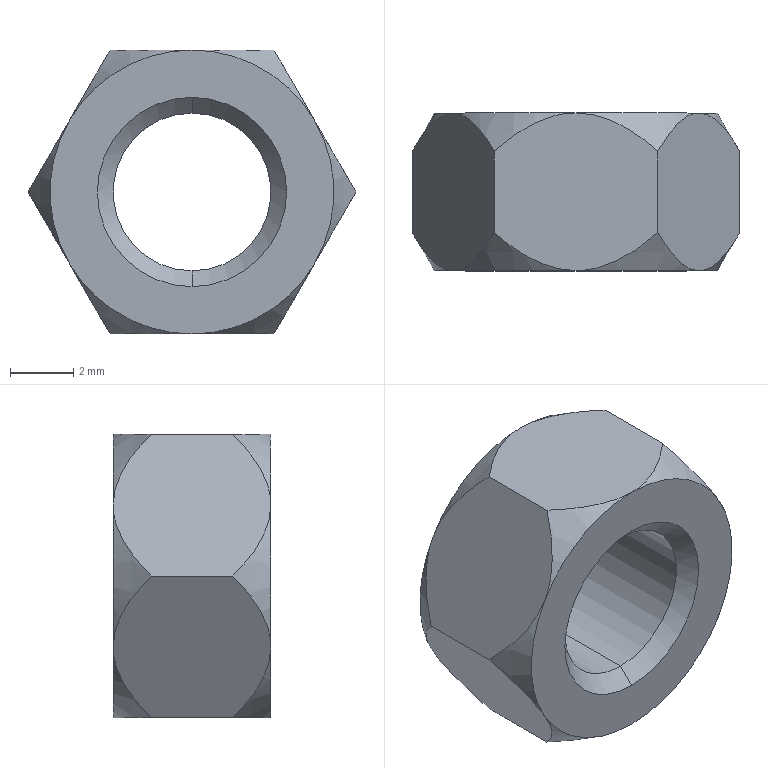Part | SolidWorks | features ICE 3, Chamfer 2, Extrusion 1 | 1 solid | 26 faces | box 10.392 x 5 x 9 mm | volume 243.63 mm3 | cone 16 | plane 8 | cylinder 2 | commonest cylinder face diameters 5 x2
STEP:
#1=CARTESIAN_POINT('',(0.,0.5,2.5));
#2=VERTEX_POINT('',#1);
#3=CARTESIAN_POINT('',(0.,0.5,-2.5));
#4=VERTEX_POINT('',#3);
#5=CARTESIAN_POINT('',(0.,0.5,0.));
#6=DIRECTION('',(0.,-1.,0.));
#7=DIRECTION('',(0.,0.,1.));
#8=AXIS2_PLACEMENT_3D('',#5,#6,#7);
#9=CIRCLE('',#8,2.5);
#10=EDGE_CURVE('',#2,#4,#9,.T.);
#11=ORIENTED_EDGE('',*,*,#10,.F.);
#12=CARTESIAN_POINT('',(0.,0.,3.));
#13=VERTEX_POINT('',#12);
#14=CARTESIAN_POINT('',(0.,0.,3.));
#15=DIRECTION('',(0.,-0.7071,0.7071));
#16=VECTOR('',#15,1000.);
#17=LINE('',#14,#16);
#18=EDGE_CURVE('',#2,#13,#17,.T.);
#19=ORIENTED_EDGE('',*,*,#18,.T.);
#20=CARTESIAN_POINT('',(0.,0.,-3.));
#21=VERTEX_POINT('',#20);
#22=CARTESIAN_POINT('',(0.,0.,0.));
#23=DIRECTION('',(0.,1.,0.));
#24=DIRECTION('',(0.,0.,1.));
#25=AXIS2_PLACEMENT_3D('',#22,#23,#24);
#26=CIRCLE('',#25,3.);
#27=EDGE_CURVE('',#21,#13,#26,.T.);
#28=ORIENTED_EDGE('',*,*,#27,.F.);
#29=CARTESIAN_POINT('',(0.,0.,-3.));
#30=DIRECTION('',(0.,-0.7071,-0.7071));
#31=VECTOR('',#30,1000.);
#32=LINE('',#29,#31);
#33=EDGE_CURVE('',#4,#21,#32,.T.);
#34=ORIENTED_EDGE('',*,*,#33,.F.);
#35=EDGE_LOOP('',(#11,#19,#28,#34));
#36=FACE_OUTER_BOUND('',#35,.T.);
#37=CARTESIAN_POINT('',(0.,0.,0.));
#38=DIRECTION('',(0.,-1.,0.));
#39=DIRECTION('',(0.,0.,-1.));
#40=AXIS2_PLACEMENT_3D('',#37,#38,#39);
#41=CONICAL_SURFACE('',#40,3.,0.7854);
#42=ADVANCED_FACE('',(#36),#41,.F.);
#43=CARTESIAN_POINT('',(0.,4.5,-2.5));
#44=VERTEX_POINT('',#43);
#45=CARTESIAN_POINT('',(0.,4.5,2.5));
#46=VERTEX_POINT('',#45);
#47=CARTESIAN_POINT('',(0.,4.5,0.));
#48=DIRECTION('',(0.,1.,0.));
#49=DIRECTION('',(0.,0.,1.));
#50=AXIS2_PLACEMENT_3D('',#47,#48,#49);
#51=CIRCLE('',#50,2.5);
#52=EDGE_CURVE('',#44,#46,#51,.T.);
#53=ORIENTED_EDGE('',*,*,#52,.F.);
#54=CARTESIAN_POINT('',(0.,5.,-3.));
#55=VERTEX_POINT('',#54);
#56=CARTESIAN_POINT('',(0.,4.5,-2.5));
#57=DIRECTION('',(0.,0.7071,-0.7071));
#58=VECTOR('',#57,1000.);
#59=LINE('',#56,#58);
#60=EDGE_CURVE('',#44,#55,#59,.T.);
#61=ORIENTED_EDGE('',*,*,#60,.T.);
#62=CARTESIAN_POINT('',(0.,5.,3.));
#63=VERTEX_POINT('',#62);
#64=CARTESIAN_POINT('',(0.,5.,0.));
#65=DIRECTION('',(0.,-1.,0.));
#66=DIRECTION('',(0.,0.,1.));
#67=AXIS2_PLACEMENT_3D('',#64,#65,#66);
#68=CIRCLE('',#67,3.);
#69=EDGE_CURVE('',#63,#55,#68,.T.);
#70=ORIENTED_EDGE('',*,*,#69,.F.);
#71=CARTESIAN_POINT('',(0.,4.5,2.5));
#72=DIRECTION('',(0.,0.7071,0.7071));
#73=VECTOR('',#72,1000.);
#74=LINE('',#71,#73);
#75=EDGE_CURVE('',#46,#63,#74,.T.);
#76=ORIENTED_EDGE('',*,*,#75,.F.);
#77=EDGE_LOOP('',(#53,#61,#70,#76));
#78=FACE_OUTER_BOUND('',#77,.T.);
#79=CARTESIAN_POINT('',(0.,4.5,0.));
#80=DIRECTION('',(0.,1.,0.));
#81=DIRECTION('',(0.,0.,1.));
#82=AXIS2_PLACEMENT_3D('',#79,#80,#81);
#83=CONICAL_SURFACE('',#82,2.5,0.7854);
#84=ADVANCED_FACE('',(#78),#83,.F.);
#85=ORIENTED_EDGE('',*,*,#10,.T.);
#86=CARTESIAN_POINT('',(0.,0.,-2.5));
#87=DIRECTION('',(0.,1.,0.));
#88=VECTOR('',#87,1000.);
#89=LINE('',#86,#88);
#90=EDGE_CURVE('',#4,#44,#89,.T.);
#91=ORIENTED_EDGE('',*,*,#90,.T.);
#92=ORIENTED_EDGE('',*,*,#52,.T.);
#93=CARTESIAN_POINT('',(0.,0.,2.5));
#94=DIRECTION('',(0.,1.,0.));
#95=VECTOR('',#94,1000.);
#96=LINE('',#93,#95);
#97=EDGE_CURVE('',#2,#46,#96,.T.);
#98=ORIENTED_EDGE('',*,*,#97,.F.);
#99=EDGE_LOOP('',(#85,#91,#92,#98));
#100=FACE_OUTER_BOUND('',#99,.T.);
#101=CARTESIAN_POINT('',(0.,0.,0.));
#102=DIRECTION('',(0.,1.,0.));
#103=DIRECTION('',(0.,0.,1.));
#104=AXIS2_PLACEMENT_3D('',#101,#102,#103);
#105=CYLINDRICAL_SURFACE('',#104,2.5);
#106=ADVANCED_FACE('',(#100),#105,.F.);
#107=CARTESIAN_POINT('',(2.598,1.206,-4.5));
#108=VERTEX_POINT('',#107);
#109=CARTESIAN_POINT('',(3.897,0.,-2.25));
#110=VERTEX_POINT('',#109);
#111=CARTESIAN_POINT('',(2.598,1.206,-4.5));
#112=CARTESIAN_POINT('',(2.783,0.8857,-4.18));
#113=CARTESIAN_POINT('',(2.978,0.5954,-3.843));
#114=CARTESIAN_POINT('',(3.302,0.2598,-3.28));
#115=CARTESIAN_POINT('',(3.417,0.1653,-3.081));
#116=CARTESIAN_POINT('',(3.593,0.06822,-2.776));
#117=CARTESIAN_POINT('',(3.653,0.04302,-2.673));
#118=CARTESIAN_POINT('',(3.774,0.00883,-2.463));
#119=CARTESIAN_POINT('',(3.836,0.,-2.356));
#120=CARTESIAN_POINT('',(3.897,0.,-2.25));
#121=B_SPLINE_CURVE_WITH_KNOTS('',3,(#111,#112,#113,#114,#115,#116,#117,#118,#119,#120),.UNSPECIFIED.,.F.,.F.,(4,2,2,2,4),(0.000000303,0.001454,0.002182,0.002545,0.002909),.UNSPECIFIED.);
#122=EDGE_CURVE('',#108,#110,#121,.T.);
#123=ORIENTED_EDGE('',*,*,#122,.F.);
#124=CARTESIAN_POINT('',(2.598,3.794,-4.5));
#125=VERTEX_POINT('',#124);
#126=CARTESIAN_POINT('',(2.598,5.,-4.5));
#127=DIRECTION('',(0.,-1.,0.));
#128=VECTOR('',#127,1000.);
#129=LINE('',#126,#128);
#130=EDGE_CURVE('',#125,#108,#129,.T.);
#131=ORIENTED_EDGE('',*,*,#130,.F.);
#132=CARTESIAN_POINT('',(3.897,5.,-2.25));
#133=VERTEX_POINT('',#132);
#134=CARTESIAN_POINT('',(3.897,5.,-2.25));
#135=CARTESIAN_POINT('',(3.775,5.,-2.461));
#136=CARTESIAN_POINT('',(3.655,4.966,-2.669));
#137=CARTESIAN_POINT('',(3.418,4.836,-3.08));
#138=CARTESIAN_POINT('',(3.305,4.743,-3.275));
#139=CARTESIAN_POINT('',(3.089,4.521,-3.649));
#140=CARTESIAN_POINT('',(2.986,4.39,-3.829));
#141=CARTESIAN_POINT('',(2.786,4.107,-4.174));
#142=CARTESIAN_POINT('',(2.691,3.955,-4.34));
#143=CARTESIAN_POINT('',(2.598,3.794,-4.5));
#144=B_SPLINE_CURVE_WITH_KNOTS('',3,(#134,#135,#136,#137,#138,#139,#140,#141,#142,#143),.UNSPECIFIED.,.F.,.F.,(4,2,2,2,4),(0.002909,0.003635,0.00436,0.005086,0.005812),.UNSPECIFIED.);
#145=EDGE_CURVE('',#133,#125,#144,.T.);
#146=ORIENTED_EDGE('',*,*,#145,.F.);
#147=CARTESIAN_POINT('',(5.196,3.794,0.));
#148=VERTEX_POINT('',#147);
#149=CARTESIAN_POINT('',(5.196,3.794,0.));
#150=CARTESIAN_POINT('',(5.011,4.114,-0.3201));
#151=CARTESIAN_POINT('',(4.817,4.405,-0.6572));
#152=CARTESIAN_POINT('',(4.492,4.74,-1.22));
#153=CARTESIAN_POINT('',(4.377,4.835,-1.419));
#154=CARTESIAN_POINT('',(4.201,4.932,-1.724));
#155=CARTESIAN_POINT('',(4.141,4.957,-1.827));
#156=CARTESIAN_POINT('',(4.02,4.991,-2.037));
#157=CARTESIAN_POINT('',(3.958,5.,-2.144));
#158=CARTESIAN_POINT('',(3.897,5.,-2.25));
#159=B_SPLINE_CURVE_WITH_KNOTS('',3,(#149,#150,#151,#152,#153,#154,#155,#156,#157,#158),.UNSPECIFIED.,.F.,.F.,(4,2,2,2,4),(0.000000303,0.001454,0.002182,0.002545,0.002909),.UNSPECIFIED.);
#160=EDGE_CURVE('',#148,#133,#159,.T.);
#161=ORIENTED_EDGE('',*,*,#160,.F.);
#162=CARTESIAN_POINT('',(5.196,1.206,0.));
#163=VERTEX_POINT('',#162);
#164=CARTESIAN_POINT('',(5.196,5.,0.));
#165=DIRECTION('',(0.,-1.,0.));
#166=VECTOR('',#165,1000.);
#167=LINE('',#164,#166);
#168=EDGE_CURVE('',#148,#163,#167,.T.);
#169=ORIENTED_EDGE('',*,*,#168,.T.);
#170=CARTESIAN_POINT('',(3.897,0.,-2.25));
#171=CARTESIAN_POINT('',(4.019,0.,-2.039));
#172=CARTESIAN_POINT('',(4.139,0.03447,-1.831));
#173=CARTESIAN_POINT('',(4.376,0.1645,-1.42));
#174=CARTESIAN_POINT('',(4.489,0.2573,-1.225));
#175=CARTESIAN_POINT('',(4.705,0.4793,-0.8509));
#176=CARTESIAN_POINT('',(4.809,0.6095,-0.6711));
#177=CARTESIAN_POINT('',(5.008,0.8928,-0.3256));
#178=CARTESIAN_POINT('',(5.104,1.045,-0.1603));
#179=CARTESIAN_POINT('',(5.196,1.206,0.));
#180=B_SPLINE_CURVE_WITH_KNOTS('',3,(#170,#171,#172,#173,#174,#175,#176,#177,#178,#179),.UNSPECIFIED.,.F.,.F.,(4,2,2,2,4),(0.002909,0.003635,0.00436,0.005086,0.005812),.UNSPECIFIED.);
#181=EDGE_CURVE('',#110,#163,#180,.T.);
#182=ORIENTED_EDGE('',*,*,#181,.F.);
#183=EDGE_LOOP('',(#123,#131,#146,#161,#169,#182));
#184=FACE_OUTER_BOUND('',#183,.T.);
#185=CARTESIAN_POINT('',(5.196,5.,0.));
#186=DIRECTION('',(-0.866,0.,0.5));
#187=DIRECTION('',(0.5,0.,0.866));
#188=AXIS2_PLACEMENT_3D('',#185,#186,#187);
#189=PLANE('',#188);
#190=ADVANCED_FACE('',(#184),#189,.F.);
#191=CARTESIAN_POINT('',(-2.598,1.206,-4.5));
#192=VERTEX_POINT('',#191);
#193=CARTESIAN_POINT('',(0.,0.,-4.5));
#194=VERTEX_POINT('',#193);
#195=CARTESIAN_POINT('',(-2.598,1.206,-4.5));
#196=CARTESIAN_POINT('',(-2.229,0.8859,-4.5));
#197=CARTESIAN_POINT('',(-1.838,0.5947,-4.5));
#198=CARTESIAN_POINT('',(-1.19,0.2599,-4.5));
#199=CARTESIAN_POINT('',(-0.9599,0.1652,-4.5));
#200=CARTESIAN_POINT('',(-0.6075,0.06813,-4.5));
#201=CARTESIAN_POINT('',(-0.4883,0.04298,-4.5));
#202=CARTESIAN_POINT('',(-0.2464,0.008879,-4.5));
#203=CARTESIAN_POINT('',(-0.1225,0.,-4.5));
#204=CARTESIAN_POINT('',(0.,0.,-4.5));
#205=B_SPLINE_CURVE_WITH_KNOTS('',3,(#195,#196,#197,#198,#199,#200,#201,#202,#203,#204),.UNSPECIFIED.,.F.,.F.,(4,2,2,2,4),(0.01211,0.01357,0.01431,0.01467,0.01504),.UNSPECIFIED.);
#206=EDGE_CURVE('',#192,#194,#205,.T.);
#207=ORIENTED_EDGE('',*,*,#206,.F.);
#208=CARTESIAN_POINT('',(-2.598,3.794,-4.5));
#209=VERTEX_POINT('',#208);
#210=CARTESIAN_POINT('',(-2.598,5.,-4.5));
#211=DIRECTION('',(0.,-1.,0.));
#212=VECTOR('',#211,1000.);
#213=LINE('',#210,#212);
#214=EDGE_CURVE('',#209,#192,#213,.T.);
#215=ORIENTED_EDGE('',*,*,#214,.F.);
#216=CARTESIAN_POINT('',(0.,5.,-4.5));
#217=VERTEX_POINT('',#216);
#218=CARTESIAN_POINT('',(0.,5.,-4.5));
#219=CARTESIAN_POINT('',(-0.2451,5.,-4.5));
#220=CARTESIAN_POINT('',(-0.4858,4.965,-4.5));
#221=CARTESIAN_POINT('',(-0.9596,4.835,-4.5));
#222=CARTESIAN_POINT('',(-1.187,4.741,-4.5));
#223=CARTESIAN_POINT('',(-1.619,4.519,-4.5));
#224=CARTESIAN_POINT('',(-1.827,4.388,-4.5));
#225=CARTESIAN_POINT('',(-2.226,4.105,-4.5));
#226=CARTESIAN_POINT('',(-2.415,3.953,-4.5));
#227=CARTESIAN_POINT('',(-2.598,3.794,-4.5));
#228=B_SPLINE_CURVE_WITH_KNOTS('',3,(#218,#219,#220,#221,#222,#223,#224,#225,#226,#227),.UNSPECIFIED.,.F.,.F.,(4,2,2,2,4),(0.01504,0.01577,0.0165,0.01723,0.01796),.UNSPECIFIED.);
#229=EDGE_CURVE('',#217,#209,#228,.T.);
#230=ORIENTED_EDGE('',*,*,#229,.F.);
#231=CARTESIAN_POINT('',(2.598,3.794,-4.5));
#232=CARTESIAN_POINT('',(2.229,4.114,-4.5));
#233=CARTESIAN_POINT('',(1.838,4.405,-4.5));
#234=CARTESIAN_POINT('',(1.19,4.74,-4.5));
#235=CARTESIAN_POINT('',(0.9599,4.835,-4.5));
#236=CARTESIAN_POINT('',(0.6075,4.932,-4.5));
#237=CARTESIAN_POINT('',(0.4883,4.957,-4.5));
#238=CARTESIAN_POINT('',(0.2464,4.991,-4.5));
#239=CARTESIAN_POINT('',(0.1225,5.,-4.5));
#240=CARTESIAN_POINT('',(0.,5.,-4.5));
#241=B_SPLINE_CURVE_WITH_KNOTS('',3,(#231,#232,#233,#234,#235,#236,#237,#238,#239,#240),.UNSPECIFIED.,.F.,.F.,(4,2,2,2,4),(0.01211,0.01357,0.01431,0.01467,0.01504),.UNSPECIFIED.);
#242=EDGE_CURVE('',#125,#217,#241,.T.);
#243=ORIENTED_EDGE('',*,*,#242,.F.);
#244=ORIENTED_EDGE('',*,*,#130,.T.);
#245=CARTESIAN_POINT('',(0.,0.,-4.5));
#246=CARTESIAN_POINT('',(0.2451,0.,-4.5));
#247=CARTESIAN_POINT('',(0.4858,0.03482,-4.5));
#248=CARTESIAN_POINT('',(0.9596,0.1649,-4.5));
#249=CARTESIAN_POINT('',(1.187,0.2586,-4.5));
#250=CARTESIAN_POINT('',(1.619,0.4814,-4.5));
#251=CARTESIAN_POINT('',(1.827,0.6118,-4.5));
#252=CARTESIAN_POINT('',(2.226,0.8955,-4.5));
#253=CARTESIAN_POINT('',(2.415,1.047,-4.5));
#254=CARTESIAN_POINT('',(2.598,1.206,-4.5));
#255=B_SPLINE_CURVE_WITH_KNOTS('',3,(#245,#246,#247,#248,#249,#250,#251,#252,#253,#254),.UNSPECIFIED.,.F.,.F.,(4,2,2,2,4),(0.01504,0.01577,0.0165,0.01723,0.01796),.UNSPECIFIED.);
#256=EDGE_CURVE('',#194,#108,#255,.T.);
#257=ORIENTED_EDGE('',*,*,#256,.F.);
#258=EDGE_LOOP('',(#207,#215,#230,#243,#244,#257));
#259=FACE_OUTER_BOUND('',#258,.T.);
#260=CARTESIAN_POINT('',(2.598,5.,-4.5));
#261=DIRECTION('',(0.,0.,1.));
#262=DIRECTION('',(1.,0.,0.));
#263=AXIS2_PLACEMENT_3D('',#260,#261,#262);
#264=PLANE('',#263);
#265=ADVANCED_FACE('',(#259),#264,.F.);
#266=CARTESIAN_POINT('',(-5.196,1.206,0.));
#267=VERTEX_POINT('',#266);
#268=CARTESIAN_POINT('',(-3.897,0.,-2.25));
#269=VERTEX_POINT('',#268);
#270=CARTESIAN_POINT('',(-5.196,1.206,0.));
#271=CARTESIAN_POINT('',(-5.011,0.8857,-0.3201));
#272=CARTESIAN_POINT('',(-4.817,0.5954,-0.6572));
#273=CARTESIAN_POINT('',(-4.492,0.2598,-1.22));
#274=CARTESIAN_POINT('',(-4.377,0.1653,-1.419));
#275=CARTESIAN_POINT('',(-4.201,0.06822,-1.724));
#276=CARTESIAN_POINT('',(-4.141,0.04302,-1.827));
#277=CARTESIAN_POINT('',(-4.02,0.00883,-2.037));
#278=CARTESIAN_POINT('',(-3.958,0.,-2.144));
#279=CARTESIAN_POINT('',(-3.897,0.,-2.25));
#280=B_SPLINE_CURVE_WITH_KNOTS('',3,(#270,#271,#272,#273,#274,#275,#276,#277,#278,#279),.UNSPECIFIED.,.F.,.F.,(4,2,2,2,4),(0.000000303,0.001454,0.002182,0.002545,0.002909),.UNSPECIFIED.);
#281=EDGE_CURVE('',#267,#269,#280,.T.);
#282=ORIENTED_EDGE('',*,*,#281,.F.);
#283=CARTESIAN_POINT('',(-5.196,3.794,0.));
#284=VERTEX_POINT('',#283);
#285=CARTESIAN_POINT('',(-5.196,5.,0.));
#286=DIRECTION('',(0.,-1.,0.));
#287=VECTOR('',#286,1000.);
#288=LINE('',#285,#287);
#289=EDGE_CURVE('',#284,#267,#288,.T.);
#290=ORIENTED_EDGE('',*,*,#289,.F.);
#291=CARTESIAN_POINT('',(-3.897,5.,-2.25));
#292=VERTEX_POINT('',#291);
#293=CARTESIAN_POINT('',(-3.897,5.,-2.25));
#294=CARTESIAN_POINT('',(-4.019,5.,-2.039));
#295=CARTESIAN_POINT('',(-4.139,4.966,-1.831));
#296=CARTESIAN_POINT('',(-4.376,4.836,-1.42));
#297=CARTESIAN_POINT('',(-4.489,4.743,-1.225));
#298=CARTESIAN_POINT('',(-4.705,4.521,-0.8509));
#299=CARTESIAN_POINT('',(-4.809,4.39,-0.6711));
#300=CARTESIAN_POINT('',(-5.008,4.107,-0.3256));
#301=CARTESIAN_POINT('',(-5.104,3.955,-0.1603));
#302=CARTESIAN_POINT('',(-5.196,3.794,0.));
#303=B_SPLINE_CURVE_WITH_KNOTS('',3,(#293,#294,#295,#296,#297,#298,#299,#300,#301,#302),.UNSPECIFIED.,.F.,.F.,(4,2,2,2,4),(0.002909,0.003635,0.00436,0.005086,0.005812),.UNSPECIFIED.);
#304=EDGE_CURVE('',#292,#284,#303,.T.);
#305=ORIENTED_EDGE('',*,*,#304,.F.);
#306=CARTESIAN_POINT('',(-2.598,3.794,-4.5));
#307=CARTESIAN_POINT('',(-2.783,4.114,-4.18));
#308=CARTESIAN_POINT('',(-2.978,4.405,-3.843));
#309=CARTESIAN_POINT('',(-3.302,4.74,-3.28));
#310=CARTESIAN_POINT('',(-3.417,4.835,-3.081));
#311=CARTESIAN_POINT('',(-3.593,4.932,-2.776));
#312=CARTESIAN_POINT('',(-3.653,4.957,-2.673));
#313=CARTESIAN_POINT('',(-3.774,4.991,-2.463));
#314=CARTESIAN_POINT('',(-3.836,5.,-2.356));
#315=CARTESIAN_POINT('',(-3.897,5.,-2.25));
#316=B_SPLINE_CURVE_WITH_KNOTS('',3,(#306,#307,#308,#309,#310,#311,#312,#313,#314,#315),.UNSPECIFIED.,.F.,.F.,(4,2,2,2,4),(0.000000303,0.001454,0.002182,0.002545,0.002909),.UNSPECIFIED.);
#317=EDGE_CURVE('',#209,#292,#316,.T.);
#318=ORIENTED_EDGE('',*,*,#317,.F.);
#319=ORIENTED_EDGE('',*,*,#214,.T.);
#320=CARTESIAN_POINT('',(-3.897,0.,-2.25));
#321=CARTESIAN_POINT('',(-3.775,0.,-2.461));
#322=CARTESIAN_POINT('',(-3.655,0.03447,-2.669));
#323=CARTESIAN_POINT('',(-3.418,0.1645,-3.08));
#324=CARTESIAN_POINT('',(-3.305,0.2573,-3.275));
#325=CARTESIAN_POINT('',(-3.089,0.4793,-3.649));
#326=CARTESIAN_POINT('',(-2.986,0.6095,-3.829));
#327=CARTESIAN_POINT('',(-2.786,0.8928,-4.174));
#328=CARTESIAN_POINT('',(-2.691,1.045,-4.34));
#329=CARTESIAN_POINT('',(-2.598,1.206,-4.5));
#330=B_SPLINE_CURVE_WITH_KNOTS('',3,(#320,#321,#322,#323,#324,#325,#326,#327,#328,#329),.UNSPECIFIED.,.F.,.F.,(4,2,2,2,4),(0.002909,0.003635,0.00436,0.005086,0.005812),.UNSPECIFIED.);
#331=EDGE_CURVE('',#269,#192,#330,.T.);
#332=ORIENTED_EDGE('',*,*,#331,.F.);
#333=EDGE_LOOP('',(#282,#290,#305,#318,#319,#332));
#334=FACE_OUTER_BOUND('',#333,.T.);
#335=CARTESIAN_POINT('',(-2.598,5.,-4.5));
#336=DIRECTION('',(0.866,0.,0.5));
#337=DIRECTION('',(0.5,0.,-0.866));
#338=AXIS2_PLACEMENT_3D('',#335,#336,#337);
#339=PLANE('',#338);
#340=ADVANCED_FACE('',(#334),#339,.F.);
#341=CARTESIAN_POINT('',(-2.598,1.206,4.5));
#342=VERTEX_POINT('',#341);
#343=CARTESIAN_POINT('',(-3.897,0.,2.25));
#344=VERTEX_POINT('',#343);
#345=CARTESIAN_POINT('',(-2.598,1.206,4.5));
#346=CARTESIAN_POINT('',(-2.783,0.8857,4.18));
#347=CARTESIAN_POINT('',(-2.978,0.5954,3.843));
#348=CARTESIAN_POINT('',(-3.302,0.2598,3.28));
#349=CARTESIAN_POINT('',(-3.417,0.1653,3.081));
#350=CARTESIAN_POINT('',(-3.593,0.06822,2.776));
#351=CARTESIAN_POINT('',(-3.653,0.04302,2.673));
#352=CARTESIAN_POINT('',(-3.774,0.00883,2.463));
#353=CARTESIAN_POINT('',(-3.836,0.,2.356));
#354=CARTESIAN_POINT('',(-3.897,0.,2.25));
#355=B_SPLINE_CURVE_WITH_KNOTS('',3,(#345,#346,#347,#348,#349,#350,#351,#352,#353,#354),.UNSPECIFIED.,.F.,.F.,(4,2,2,2,4),(0.000000303,0.001454,0.002182,0.002545,0.002909),.UNSPECIFIED.);
#356=EDGE_CURVE('',#342,#344,#355,.T.);
#357=ORIENTED_EDGE('',*,*,#356,.F.);
#358=CARTESIAN_POINT('',(-2.598,3.794,4.5));
#359=VERTEX_POINT('',#358);
#360=CARTESIAN_POINT('',(-2.598,5.,4.5));
#361=DIRECTION('',(0.,-1.,0.));
#362=VECTOR('',#361,1000.);
#363=LINE('',#360,#362);
#364=EDGE_CURVE('',#359,#342,#363,.T.);
#365=ORIENTED_EDGE('',*,*,#364,.F.);
#366=CARTESIAN_POINT('',(-3.897,5.,2.25));
#367=VERTEX_POINT('',#366);
#368=CARTESIAN_POINT('',(-3.897,5.,2.25));
#369=CARTESIAN_POINT('',(-3.775,5.,2.461));
#370=CARTESIAN_POINT('',(-3.655,4.966,2.669));
#371=CARTESIAN_POINT('',(-3.418,4.836,3.08));
#372=CARTESIAN_POINT('',(-3.305,4.743,3.275));
#373=CARTESIAN_POINT('',(-3.089,4.521,3.649));
#374=CARTESIAN_POINT('',(-2.986,4.39,3.829));
#375=CARTESIAN_POINT('',(-2.786,4.107,4.174));
#376=CARTESIAN_POINT('',(-2.691,3.955,4.34));
#377=CARTESIAN_POINT('',(-2.598,3.794,4.5));
#378=B_SPLINE_CURVE_WITH_KNOTS('',3,(#368,#369,#370,#371,#372,#373,#374,#375,#376,#377),.UNSPECIFIED.,.F.,.F.,(4,2,2,2,4),(0.002909,0.003635,0.00436,0.005086,0.005812),.UNSPECIFIED.);
#379=EDGE_CURVE('',#367,#359,#378,.T.);
#380=ORIENTED_EDGE('',*,*,#379,.F.);
#381=CARTESIAN_POINT('',(-5.196,3.794,0.));
#382=CARTESIAN_POINT('',(-5.011,4.114,0.3201));
#383=CARTESIAN_POINT('',(-4.817,4.405,0.6572));
#384=CARTESIAN_POINT('',(-4.492,4.74,1.22));
#385=CARTESIAN_POINT('',(-4.377,4.835,1.419));
#386=CARTESIAN_POINT('',(-4.201,4.932,1.724));
#387=CARTESIAN_POINT('',(-4.141,4.957,1.827));
#388=CARTESIAN_POINT('',(-4.02,4.991,2.037));
#389=CARTESIAN_POINT('',(-3.958,5.,2.144));
#390=CARTESIAN_POINT('',(-3.897,5.,2.25));
#391=B_SPLINE_CURVE_WITH_KNOTS('',3,(#381,#382,#383,#384,#385,#386,#387,#388,#389,#390),.UNSPECIFIED.,.F.,.F.,(4,2,2,2,4),(0.000000303,0.001454,0.002182,0.002545,0.002909),.UNSPECIFIED.);
#392=EDGE_CURVE('',#284,#367,#391,.T.);
#393=ORIENTED_EDGE('',*,*,#392,.F.);
#394=ORIENTED_EDGE('',*,*,#289,.T.);
#395=CARTESIAN_POINT('',(-3.897,0.,2.25));
#396=CARTESIAN_POINT('',(-4.019,0.,2.039));
#397=CARTESIAN_POINT('',(-4.139,0.03447,1.831));
#398=CARTESIAN_POINT('',(-4.376,0.1645,1.42));
#399=CARTESIAN_POINT('',(-4.489,0.2573,1.225));
#400=CARTESIAN_POINT('',(-4.705,0.4793,0.8509));
#401=CARTESIAN_POINT('',(-4.809,0.6095,0.6711));
#402=CARTESIAN_POINT('',(-5.008,0.8928,0.3256));
#403=CARTESIAN_POINT('',(-5.104,1.045,0.1603));
#404=CARTESIAN_POINT('',(-5.196,1.206,0.));
#405=B_SPLINE_CURVE_WITH_KNOTS('',3,(#395,#396,#397,#398,#399,#400,#401,#402,#403,#404),.UNSPECIFIED.,.F.,.F.,(4,2,2,2,4),(0.002909,0.003635,0.00436,0.005086,0.005812),.UNSPECIFIED.);
#406=EDGE_CURVE('',#344,#267,#405,.T.);
#407=ORIENTED_EDGE('',*,*,#406,.F.);
#408=EDGE_LOOP('',(#357,#365,#380,#393,#394,#407));
#409=FACE_OUTER_BOUND('',#408,.T.);
#410=CARTESIAN_POINT('',(-5.196,5.,0.));
#411=DIRECTION('',(0.866,0.,-0.5));
#412=DIRECTION('',(-0.5,0.,-0.866));
#413=AXIS2_PLACEMENT_3D('',#410,#411,#412);
#414=PLANE('',#413);
#415=ADVANCED_FACE('',(#409),#414,.F.);
#416=CARTESIAN_POINT('',(2.598,1.206,4.5));
#417=VERTEX_POINT('',#416);
#418=CARTESIAN_POINT('',(0.,0.,4.5));
#419=VERTEX_POINT('',#418);
#420=CARTESIAN_POINT('',(2.598,1.206,4.5));
#421=CARTESIAN_POINT('',(2.229,0.8859,4.5));
#422=CARTESIAN_POINT('',(1.838,0.5947,4.5));
#423=CARTESIAN_POINT('',(1.19,0.2599,4.5));
#424=CARTESIAN_POINT('',(0.9599,0.1652,4.5));
#425=CARTESIAN_POINT('',(0.6075,0.06813,4.5));
#426=CARTESIAN_POINT('',(0.4883,0.04298,4.5));
#427=CARTESIAN_POINT('',(0.2464,0.008879,4.5));
#428=CARTESIAN_POINT('',(0.1225,0.,4.5));
#429=CARTESIAN_POINT('',(0.,0.,4.5));
#430=B_SPLINE_CURVE_WITH_KNOTS('',3,(#420,#421,#422,#423,#424,#425,#426,#427,#428,#429),.UNSPECIFIED.,.F.,.F.,(4,2,2,2,4),(0.01211,0.01357,0.01431,0.01467,0.01504),.UNSPECIFIED.);
#431=EDGE_CURVE('',#417,#419,#430,.T.);
#432=ORIENTED_EDGE('',*,*,#431,.F.);
#433=CARTESIAN_POINT('',(2.598,3.794,4.5));
#434=VERTEX_POINT('',#433);
#435=CARTESIAN_POINT('',(2.598,5.,4.5));
#436=DIRECTION('',(0.,-1.,0.));
#437=VECTOR('',#436,1000.);
#438=LINE('',#435,#437);
#439=EDGE_CURVE('',#434,#417,#438,.T.);
#440=ORIENTED_EDGE('',*,*,#439,.F.);
#441=CARTESIAN_POINT('',(0.,5.,4.5));
#442=VERTEX_POINT('',#441);
#443=CARTESIAN_POINT('',(0.,5.,4.5));
#444=CARTESIAN_POINT('',(0.2451,5.,4.5));
#445=CARTESIAN_POINT('',(0.4858,4.965,4.5));
#446=CARTESIAN_POINT('',(0.9596,4.835,4.5));
#447=CARTESIAN_POINT('',(1.187,4.741,4.5));
#448=CARTESIAN_POINT('',(1.619,4.519,4.5));
#449=CARTESIAN_POINT('',(1.827,4.388,4.5));
#450=CARTESIAN_POINT('',(2.226,4.105,4.5));
#451=CARTESIAN_POINT('',(2.415,3.953,4.5));
#452=CARTESIAN_POINT('',(2.598,3.794,4.5));
#453=B_SPLINE_CURVE_WITH_KNOTS('',3,(#443,#444,#445,#446,#447,#448,#449,#450,#451,#452),.UNSPECIFIED.,.F.,.F.,(4,2,2,2,4),(0.01504,0.01577,0.0165,0.01723,0.01796),.UNSPECIFIED.);
#454=EDGE_CURVE('',#442,#434,#453,.T.);
#455=ORIENTED_EDGE('',*,*,#454,.F.);
#456=CARTESIAN_POINT('',(-2.598,3.794,4.5));
#457=CARTESIAN_POINT('',(-2.229,4.114,4.5));
#458=CARTESIAN_POINT('',(-1.838,4.405,4.5));
#459=CARTESIAN_POINT('',(-1.19,4.74,4.5));
#460=CARTESIAN_POINT('',(-0.9599,4.835,4.5));
#461=CARTESIAN_POINT('',(-0.6075,4.932,4.5));
#462=CARTESIAN_POINT('',(-0.4883,4.957,4.5));
#463=CARTESIAN_POINT('',(-0.2464,4.991,4.5));
#464=CARTESIAN_POINT('',(-0.1225,5.,4.5));
#465=CARTESIAN_POINT('',(0.,5.,4.5));
#466=B_SPLINE_CURVE_WITH_KNOTS('',3,(#456,#457,#458,#459,#460,#461,#462,#463,#464,#465),.UNSPECIFIED.,.F.,.F.,(4,2,2,2,4),(0.01211,0.01357,0.01431,0.01467,0.01504),.UNSPECIFIED.);
#467=EDGE_CURVE('',#359,#442,#466,.T.);
#468=ORIENTED_EDGE('',*,*,#467,.F.);
#469=ORIENTED_EDGE('',*,*,#364,.T.);
#470=CARTESIAN_POINT('',(0.,0.,4.5));
#471=CARTESIAN_POINT('',(-0.2451,0.,4.5));
#472=CARTESIAN_POINT('',(-0.4858,0.03482,4.5));
#473=CARTESIAN_POINT('',(-0.9596,0.1649,4.5));
#474=CARTESIAN_POINT('',(-1.187,0.2586,4.5));
#475=CARTESIAN_POINT('',(-1.619,0.4814,4.5));
#476=CARTESIAN_POINT('',(-1.827,0.6118,4.5));
#477=CARTESIAN_POINT('',(-2.226,0.8955,4.5));
#478=CARTESIAN_POINT('',(-2.415,1.047,4.5));
#479=CARTESIAN_POINT('',(-2.598,1.206,4.5));
#480=B_SPLINE_CURVE_WITH_KNOTS('',3,(#470,#471,#472,#473,#474,#475,#476,#477,#478,#479),.UNSPECIFIED.,.F.,.F.,(4,2,2,2,4),(0.01504,0.01577,0.0165,0.01723,0.01796),.UNSPECIFIED.);
#481=EDGE_CURVE('',#419,#342,#480,.T.);
#482=ORIENTED_EDGE('',*,*,#481,.F.);
#483=EDGE_LOOP('',(#432,#440,#455,#468,#469,#482));
#484=FACE_OUTER_BOUND('',#483,.T.);
#485=CARTESIAN_POINT('',(-2.598,5.,4.5));
#486=DIRECTION('',(0.,0.,-1.));
#487=DIRECTION('',(-1.,0.,0.));
#488=AXIS2_PLACEMENT_3D('',#485,#486,#487);
#489=PLANE('',#488);
#490=ADVANCED_FACE('',(#484),#489,.F.);
#491=CARTESIAN_POINT('',(3.897,0.,2.25));
#492=VERTEX_POINT('',#491);
#493=CARTESIAN_POINT('',(5.196,1.206,0.));
#494=CARTESIAN_POINT('',(5.011,0.8857,0.3201));
#495=CARTESIAN_POINT('',(4.817,0.5954,0.6572));
#496=CARTESIAN_POINT('',(4.492,0.2598,1.22));
#497=CARTESIAN_POINT('',(4.377,0.1653,1.419));
#498=CARTESIAN_POINT('',(4.201,0.06822,1.724));
#499=CARTESIAN_POINT('',(4.141,0.04302,1.827));
#500=CARTESIAN_POINT('',(4.02,0.00883,2.037));
#501=CARTESIAN_POINT('',(3.958,0.,2.144));
#502=CARTESIAN_POINT('',(3.897,0.,2.25));
#503=B_SPLINE_CURVE_WITH_KNOTS('',3,(#493,#494,#495,#496,#497,#498,#499,#500,#501,#502),.UNSPECIFIED.,.F.,.F.,(4,2,2,2,4),(0.000000303,0.001454,0.002182,0.002545,0.002909),.UNSPECIFIED.);
#504=EDGE_CURVE('',#163,#492,#503,.T.);
#505=ORIENTED_EDGE('',*,*,#504,.F.);
#506=ORIENTED_EDGE('',*,*,#168,.F.);
#507=CARTESIAN_POINT('',(3.897,5.,2.25));
#508=VERTEX_POINT('',#507);
#509=CARTESIAN_POINT('',(3.897,5.,2.25));
#510=CARTESIAN_POINT('',(4.019,5.,2.039));
#511=CARTESIAN_POINT('',(4.139,4.966,1.831));
#512=CARTESIAN_POINT('',(4.376,4.836,1.42));
#513=CARTESIAN_POINT('',(4.489,4.743,1.225));
#514=CARTESIAN_POINT('',(4.705,4.521,0.8509));
#515=CARTESIAN_POINT('',(4.809,4.39,0.6711));
#516=CARTESIAN_POINT('',(5.008,4.107,0.3256));
#517=CARTESIAN_POINT('',(5.104,3.955,0.1603));
#518=CARTESIAN_POINT('',(5.196,3.794,0.));
#519=B_SPLINE_CURVE_WITH_KNOTS('',3,(#509,#510,#511,#512,#513,#514,#515,#516,#517,#518),.UNSPECIFIED.,.F.,.F.,(4,2,2,2,4),(0.002909,0.003635,0.00436,0.005086,0.005812),.UNSPECIFIED.);
#520=EDGE_CURVE('',#508,#148,#519,.T.);
#521=ORIENTED_EDGE('',*,*,#520,.F.);
#522=CARTESIAN_POINT('',(2.598,3.794,4.5));
#523=CARTESIAN_POINT('',(2.783,4.114,4.18));
#524=CARTESIAN_POINT('',(2.978,4.405,3.843));
#525=CARTESIAN_POINT('',(3.302,4.74,3.28));
#526=CARTESIAN_POINT('',(3.417,4.835,3.081));
#527=CARTESIAN_POINT('',(3.593,4.932,2.776));
#528=CARTESIAN_POINT('',(3.653,4.957,2.673));
#529=CARTESIAN_POINT('',(3.774,4.991,2.463));
#530=CARTESIAN_POINT('',(3.836,5.,2.356));
#531=CARTESIAN_POINT('',(3.897,5.,2.25));
#532=B_SPLINE_CURVE_WITH_KNOTS('',3,(#522,#523,#524,#525,#526,#527,#528,#529,#530,#531),.UNSPECIFIED.,.F.,.F.,(4,2,2,2,4),(0.000000303,0.001454,0.002182,0.002545,0.002909),.UNSPECIFIED.);
#533=EDGE_CURVE('',#434,#508,#532,.T.);
#534=ORIENTED_EDGE('',*,*,#533,.F.);
#535=ORIENTED_EDGE('',*,*,#439,.T.);
#536=CARTESIAN_POINT('',(3.897,0.,2.25));
#537=CARTESIAN_POINT('',(3.775,0.,2.461));
#538=CARTESIAN_POINT('',(3.655,0.03447,2.669));
#539=CARTESIAN_POINT('',(3.418,0.1645,3.08));
#540=CARTESIAN_POINT('',(3.305,0.2573,3.275));
#541=CARTESIAN_POINT('',(3.089,0.4793,3.649));
#542=CARTESIAN_POINT('',(2.986,0.6095,3.829));
#543=CARTESIAN_POINT('',(2.786,0.8928,4.174));
#544=CARTESIAN_POINT('',(2.691,1.045,4.34));
#545=CARTESIAN_POINT('',(2.598,1.206,4.5));
#546=B_SPLINE_CURVE_WITH_KNOTS('',3,(#536,#537,#538,#539,#540,#541,#542,#543,#544,#545),.UNSPECIFIED.,.F.,.F.,(4,2,2,2,4),(0.002909,0.003635,0.00436,0.005086,0.005812),.UNSPECIFIED.);
#547=EDGE_CURVE('',#492,#417,#546,.T.);
#548=ORIENTED_EDGE('',*,*,#547,.F.);
#549=EDGE_LOOP('',(#505,#506,#521,#534,#535,#548));
#550=FACE_OUTER_BOUND('',#549,.T.);
#551=CARTESIAN_POINT('',(2.598,5.,4.5));
#552=DIRECTION('',(-0.866,0.,-0.5));
#553=DIRECTION('',(-0.5,0.,0.866));
#554=AXIS2_PLACEMENT_3D('',#551,#552,#553);
#555=PLANE('',#554);
#556=ADVANCED_FACE('',(#550),#555,.F.);
#557=ORIENTED_EDGE('',*,*,#27,.T.);
#558=CARTESIAN_POINT('',(0.,0.,0.));
#559=DIRECTION('',(0.,1.,0.));
#560=DIRECTION('',(0.,0.,1.));
#561=AXIS2_PLACEMENT_3D('',#558,#559,#560);
#562=CIRCLE('',#561,3.);
#563=EDGE_CURVE('',#13,#21,#562,.T.);
#564=ORIENTED_EDGE('',*,*,#563,.T.);
#565=EDGE_LOOP('',(#557,#564));
#566=FACE_BOUND('',#565,.T.);
#567=CARTESIAN_POINT('',(0.,0.,0.));
#568=DIRECTION('',(0.,1.,0.));
#569=DIRECTION('',(0.,0.,1.));
#570=AXIS2_PLACEMENT_3D('',#567,#568,#569);
#571=CIRCLE('',#570,4.5);
#572=EDGE_CURVE('',#419,#492,#571,.T.);
#573=ORIENTED_EDGE('',*,*,#572,.F.);
#574=CARTESIAN_POINT('',(0.,0.,0.));
#575=DIRECTION('',(0.,1.,0.));
#576=DIRECTION('',(0.,0.,1.));
#577=AXIS2_PLACEMENT_3D('',#574,#575,#576);
#578=CIRCLE('',#577,4.5);
#579=EDGE_CURVE('',#344,#419,#578,.T.);
#580=ORIENTED_EDGE('',*,*,#579,.F.);
#581=CARTESIAN_POINT('',(0.,0.,0.));
#582=DIRECTION('',(0.,1.,0.));
#583=DIRECTION('',(0.,0.,1.));
#584=AXIS2_PLACEMENT_3D('',#581,#582,#583);
#585=CIRCLE('',#584,4.5);
#586=EDGE_CURVE('',#269,#344,#585,.T.);
#587=ORIENTED_EDGE('',*,*,#586,.F.);
#588=CARTESIAN_POINT('',(0.,0.,0.));
#589=DIRECTION('',(0.,1.,0.));
#590=DIRECTION('',(0.,0.,1.));
#591=AXIS2_PLACEMENT_3D('',#588,#589,#590);
#592=CIRCLE('',#591,4.5);
#593=EDGE_CURVE('',#194,#269,#592,.T.);
#594=ORIENTED_EDGE('',*,*,#593,.F.);
#595=CARTESIAN_POINT('',(0.,0.,0.));
#596=DIRECTION('',(0.,-1.,0.));
#597=DIRECTION('',(0.,0.,-1.));
#598=AXIS2_PLACEMENT_3D('',#595,#596,#597);
#599=CIRCLE('',#598,4.5);
#600=EDGE_CURVE('',#194,#110,#599,.T.);
#601=ORIENTED_EDGE('',*,*,#600,.T.);
#602=CARTESIAN_POINT('',(0.,0.,0.));
#603=DIRECTION('',(0.,1.,0.));
#604=DIRECTION('',(0.,0.,1.));
#605=AXIS2_PLACEMENT_3D('',#602,#603,#604);
#606=CIRCLE('',#605,4.5);
#607=EDGE_CURVE('',#492,#110,#606,.T.);
#608=ORIENTED_EDGE('',*,*,#607,.F.);
#609=EDGE_LOOP('',(#573,#580,#587,#594,#601,#608));
#610=FACE_OUTER_BOUND('',#609,.T.);
#611=CARTESIAN_POINT('',(0.,0.,0.));
#612=DIRECTION('',(0.,1.,0.));
#613=DIRECTION('',(0.,0.,1.));
#614=AXIS2_PLACEMENT_3D('',#611,#612,#613);
#615=PLANE('',#614);
#616=ADVANCED_FACE('',(#566,#610),#615,.F.);
#617=ORIENTED_EDGE('',*,*,#69,.T.);
#618=CARTESIAN_POINT('',(0.,5.,0.));
#619=DIRECTION('',(0.,-1.,0.));
#620=DIRECTION('',(0.,0.,1.));
#621=AXIS2_PLACEMENT_3D('',#618,#619,#620);
#622=CIRCLE('',#621,3.);
#623=EDGE_CURVE('',#55,#63,#622,.T.);
#624=ORIENTED_EDGE('',*,*,#623,.T.);
#625=EDGE_LOOP('',(#617,#624));
#626=FACE_BOUND('',#625,.T.);
#627=CARTESIAN_POINT('',(0.,5.,0.));
#628=DIRECTION('',(0.,1.,0.));
#629=DIRECTION('',(0.,0.,1.));
#630=AXIS2_PLACEMENT_3D('',#627,#628,#629);
#631=CIRCLE('',#630,4.5);
#632=EDGE_CURVE('',#367,#442,#631,.T.);
#633=ORIENTED_EDGE('',*,*,#632,.T.);
#634=CARTESIAN_POINT('',(0.,5.,0.));
#635=DIRECTION('',(0.,1.,0.));
#636=DIRECTION('',(0.,0.,1.));
#637=AXIS2_PLACEMENT_3D('',#634,#635,#636);
#638=CIRCLE('',#637,4.5);
#639=EDGE_CURVE('',#442,#508,#638,.T.);
#640=ORIENTED_EDGE('',*,*,#639,.T.);
#641=CARTESIAN_POINT('',(0.,5.,0.));
#642=DIRECTION('',(0.,1.,0.));
#643=DIRECTION('',(0.,0.,1.));
#644=AXIS2_PLACEMENT_3D('',#641,#642,#643);
#645=CIRCLE('',#644,4.5);
#646=EDGE_CURVE('',#508,#133,#645,.T.);
#647=ORIENTED_EDGE('',*,*,#646,.T.);
#648=CARTESIAN_POINT('',(0.,5.,0.));
#649=DIRECTION('',(0.,1.,0.));
#650=DIRECTION('',(0.,0.,1.));
#651=AXIS2_PLACEMENT_3D('',#648,#649,#650);
#652=CIRCLE('',#651,4.5);
#653=EDGE_CURVE('',#133,#217,#652,.T.);
#654=ORIENTED_EDGE('',*,*,#653,.T.);
#655=CARTESIAN_POINT('',(0.,5.,0.));
#656=DIRECTION('',(0.,1.,0.));
#657=DIRECTION('',(0.,0.,1.));
#658=AXIS2_PLACEMENT_3D('',#655,#656,#657);
#659=CIRCLE('',#658,4.5);
#660=EDGE_CURVE('',#217,#292,#659,.T.);
#661=ORIENTED_EDGE('',*,*,#660,.T.);
#662=CARTESIAN_POINT('',(0.,5.,0.));
#663=DIRECTION('',(0.,1.,0.));
#664=DIRECTION('',(0.,0.,1.));
#665=AXIS2_PLACEMENT_3D('',#662,#663,#664);
#666=CIRCLE('',#665,4.5);
#667=EDGE_CURVE('',#292,#367,#666,.T.);
#668=ORIENTED_EDGE('',*,*,#667,.T.);
#669=EDGE_LOOP('',(#633,#640,#647,#654,#661,#668));
#670=FACE_OUTER_BOUND('',#669,.T.);
#671=CARTESIAN_POINT('',(0.,5.,0.));
#672=DIRECTION('',(0.,1.,0.));
#673=DIRECTION('',(0.,0.,1.));
#674=AXIS2_PLACEMENT_3D('',#671,#672,#673);
#675=PLANE('',#674);
#676=ADVANCED_FACE('',(#626,#670),#675,.T.);
#677=ORIENTED_EDGE('',*,*,#90,.F.);
#678=CARTESIAN_POINT('',(0.,0.5,0.));
#679=DIRECTION('',(0.,-1.,0.));
#680=DIRECTION('',(0.,0.,1.));
#681=AXIS2_PLACEMENT_3D('',#678,#679,#680);
#682=CIRCLE('',#681,2.5);
#683=EDGE_CURVE('',#4,#2,#682,.T.);
#684=ORIENTED_EDGE('',*,*,#683,.T.);
#685=ORIENTED_EDGE('',*,*,#97,.T.);
#686=CARTESIAN_POINT('',(0.,4.5,0.));
#687=DIRECTION('',(0.,1.,0.));
#688=DIRECTION('',(0.,0.,1.));
#689=AXIS2_PLACEMENT_3D('',#686,#687,#688);
#690=CIRCLE('',#689,2.5);
#691=EDGE_CURVE('',#46,#44,#690,.T.);
#692=ORIENTED_EDGE('',*,*,#691,.T.);
#693=EDGE_LOOP('',(#677,#684,#685,#692));
#694=FACE_OUTER_BOUND('',#693,.T.);
#695=CARTESIAN_POINT('',(0.,0.,0.));
#696=DIRECTION('',(0.,1.,0.));
#697=DIRECTION('',(0.,0.,1.));
#698=AXIS2_PLACEMENT_3D('',#695,#696,#697);
#699=CYLINDRICAL_SURFACE('',#698,2.5);
#700=ADVANCED_FACE('',(#694),#699,.F.);
#701=ORIENTED_EDGE('',*,*,#379,.T.);
#702=ORIENTED_EDGE('',*,*,#467,.T.);
#703=ORIENTED_EDGE('',*,*,#632,.F.);
#704=EDGE_LOOP('',(#701,#702,#703));
#705=FACE_OUTER_BOUND('',#704,.T.);
#706=CARTESIAN_POINT('',(0.,5.,0.));
#707=DIRECTION('',(0.,-1.,0.));
#708=DIRECTION('',(0.,0.,1.));
#709=AXIS2_PLACEMENT_3D('',#706,#707,#708);
#710=CONICAL_SURFACE('',#709,4.5,0.5236);
#711=ADVANCED_FACE('',(#705),#710,.T.);
#712=ORIENTED_EDGE('',*,*,#304,.T.);
#713=ORIENTED_EDGE('',*,*,#392,.T.);
#714=ORIENTED_EDGE('',*,*,#667,.F.);
#715=EDGE_LOOP('',(#712,#713,#714));
#716=FACE_OUTER_BOUND('',#715,.T.);
#717=CARTESIAN_POINT('',(0.,5.,0.));
#718=DIRECTION('',(0.,-1.,0.));
#719=DIRECTION('',(0.,0.,1.));
#720=AXIS2_PLACEMENT_3D('',#717,#718,#719);
#721=CONICAL_SURFACE('',#720,4.5,0.5236);
#722=ADVANCED_FACE('',(#716),#721,.T.);
#723=ORIENTED_EDGE('',*,*,#229,.T.);
#724=ORIENTED_EDGE('',*,*,#317,.T.);
#725=ORIENTED_EDGE('',*,*,#660,.F.);
#726=EDGE_LOOP('',(#723,#724,#725));
#727=FACE_OUTER_BOUND('',#726,.T.);
#728=CARTESIAN_POINT('',(0.,5.,0.));
#729=DIRECTION('',(0.,-1.,0.));
#730=DIRECTION('',(0.,0.,1.));
#731=AXIS2_PLACEMENT_3D('',#728,#729,#730);
#732=CONICAL_SURFACE('',#731,4.5,0.5236);
#733=ADVANCED_FACE('',(#727),#732,.T.);
#734=ORIENTED_EDGE('',*,*,#145,.T.);
#735=ORIENTED_EDGE('',*,*,#242,.T.);
#736=ORIENTED_EDGE('',*,*,#653,.F.);
#737=EDGE_LOOP('',(#734,#735,#736));
#738=FACE_OUTER_BOUND('',#737,.T.);
#739=CARTESIAN_POINT('',(0.,5.,0.));
#740=DIRECTION('',(0.,-1.,0.));
#741=DIRECTION('',(0.,0.,1.));
#742=AXIS2_PLACEMENT_3D('',#739,#740,#741);
#743=CONICAL_SURFACE('',#742,4.5,0.5236);
#744=ADVANCED_FACE('',(#738),#743,.T.);
#745=ORIENTED_EDGE('',*,*,#160,.T.);
#746=ORIENTED_EDGE('',*,*,#646,.F.);
#747=ORIENTED_EDGE('',*,*,#520,.T.);
#748=EDGE_LOOP('',(#745,#746,#747));
#749=FACE_OUTER_BOUND('',#748,.T.);
#750=CARTESIAN_POINT('',(0.,5.,0.));
#751=DIRECTION('',(0.,-1.,0.));
#752=DIRECTION('',(0.,0.,1.));
#753=AXIS2_PLACEMENT_3D('',#750,#751,#752);
#754=CONICAL_SURFACE('',#753,4.5,0.5236);
#755=ADVANCED_FACE('',(#749),#754,.T.);
#756=ORIENTED_EDGE('',*,*,#454,.T.);
#757=ORIENTED_EDGE('',*,*,#533,.T.);
#758=ORIENTED_EDGE('',*,*,#639,.F.);
#759=EDGE_LOOP('',(#756,#757,#758));
#760=FACE_OUTER_BOUND('',#759,.T.);
#761=CARTESIAN_POINT('',(0.,5.,0.));
#762=DIRECTION('',(0.,-1.,0.));
#763=DIRECTION('',(0.,0.,1.));
#764=AXIS2_PLACEMENT_3D('',#761,#762,#763);
#765=CONICAL_SURFACE('',#764,4.5,0.5236);
#766=ADVANCED_FACE('',(#760),#765,.T.);
#767=ORIENTED_EDGE('',*,*,#356,.T.);
#768=ORIENTED_EDGE('',*,*,#579,.T.);
#769=ORIENTED_EDGE('',*,*,#481,.T.);
#770=EDGE_LOOP('',(#767,#768,#769));
#771=FACE_OUTER_BOUND('',#770,.T.);
#772=CARTESIAN_POINT('',(0.,0.,0.));
#773=DIRECTION('',(0.,1.,0.));
#774=DIRECTION('',(0.,0.,-1.));
#775=AXIS2_PLACEMENT_3D('',#772,#773,#774);
#776=CONICAL_SURFACE('',#775,4.5,0.5236);
#777=ADVANCED_FACE('',(#771),#776,.T.);
#778=ORIENTED_EDGE('',*,*,#281,.T.);
#779=ORIENTED_EDGE('',*,*,#586,.T.);
#780=ORIENTED_EDGE('',*,*,#406,.T.);
#781=EDGE_LOOP('',(#778,#779,#780));
#782=FACE_OUTER_BOUND('',#781,.T.);
#783=CARTESIAN_POINT('',(0.,0.,0.));
#784=DIRECTION('',(0.,1.,0.));
#785=DIRECTION('',(0.,0.,-1.));
#786=AXIS2_PLACEMENT_3D('',#783,#784,#785);
#787=CONICAL_SURFACE('',#786,4.5,0.5236);
#788=ADVANCED_FACE('',(#782),#787,.T.);
#789=ORIENTED_EDGE('',*,*,#331,.T.);
#790=ORIENTED_EDGE('',*,*,#206,.T.);
#791=ORIENTED_EDGE('',*,*,#593,.T.);
#792=EDGE_LOOP('',(#789,#790,#791));
#793=FACE_OUTER_BOUND('',#792,.T.);
#794=CARTESIAN_POINT('',(0.,0.,0.));
#795=DIRECTION('',(0.,1.,0.));
#796=DIRECTION('',(0.,0.,-1.));
#797=AXIS2_PLACEMENT_3D('',#794,#795,#796);
#798=CONICAL_SURFACE('',#797,4.5,0.5236);
#799=ADVANCED_FACE('',(#793),#798,.T.);
#800=ORIENTED_EDGE('',*,*,#256,.T.);
#801=ORIENTED_EDGE('',*,*,#122,.T.);
#802=ORIENTED_EDGE('',*,*,#600,.F.);
#803=EDGE_LOOP('',(#800,#801,#802));
#804=FACE_OUTER_BOUND('',#803,.T.);
#805=CARTESIAN_POINT('',(0.,0.,0.));
#806=DIRECTION('',(0.,1.,0.));
#807=DIRECTION('',(0.,0.,-1.));
#808=AXIS2_PLACEMENT_3D('',#805,#806,#807);
#809=CONICAL_SURFACE('',#808,4.5,0.5236);
#810=ADVANCED_FACE('',(#804),#809,.T.);
#811=ORIENTED_EDGE('',*,*,#181,.T.);
#812=ORIENTED_EDGE('',*,*,#504,.T.);
#813=ORIENTED_EDGE('',*,*,#607,.T.);
#814=EDGE_LOOP('',(#811,#812,#813));
#815=FACE_OUTER_BOUND('',#814,.T.);
#816=CARTESIAN_POINT('',(0.,0.,0.));
#817=DIRECTION('',(0.,1.,0.));
#818=DIRECTION('',(0.,0.,-1.));
#819=AXIS2_PLACEMENT_3D('',#816,#817,#818);
#820=CONICAL_SURFACE('',#819,4.5,0.5236);
#821=ADVANCED_FACE('',(#815),#820,.T.);
#822=ORIENTED_EDGE('',*,*,#431,.T.);
#823=ORIENTED_EDGE('',*,*,#572,.T.);
#824=ORIENTED_EDGE('',*,*,#547,.T.);
#825=EDGE_LOOP('',(#822,#823,#824));
#826=FACE_OUTER_BOUND('',#825,.T.);
#827=CARTESIAN_POINT('',(0.,0.,0.));
#828=DIRECTION('',(0.,1.,0.));
#829=DIRECTION('',(0.,0.,-1.));
#830=AXIS2_PLACEMENT_3D('',#827,#828,#829);
#831=CONICAL_SURFACE('',#830,4.5,0.5236);
#832=ADVANCED_FACE('',(#826),#831,.T.);
#833=ORIENTED_EDGE('',*,*,#60,.F.);
#834=ORIENTED_EDGE('',*,*,#691,.F.);
#835=ORIENTED_EDGE('',*,*,#75,.T.);
#836=ORIENTED_EDGE('',*,*,#623,.F.);
#837=EDGE_LOOP('',(#833,#834,#835,#836));
#838=FACE_OUTER_BOUND('',#837,.T.);
#839=CARTESIAN_POINT('',(0.,4.5,0.));
#840=DIRECTION('',(0.,1.,0.));
#841=DIRECTION('',(0.,0.,1.));
#842=AXIS2_PLACEMENT_3D('',#839,#840,#841);
#843=CONICAL_SURFACE('',#842,2.5,0.7854);
#844=ADVANCED_FACE('',(#838),#843,.F.);
#845=ORIENTED_EDGE('',*,*,#18,.F.);
#846=ORIENTED_EDGE('',*,*,#683,.F.);
#847=ORIENTED_EDGE('',*,*,#33,.T.);
#848=ORIENTED_EDGE('',*,*,#563,.F.);
#849=EDGE_LOOP('',(#845,#846,#847,#848));
#850=FACE_OUTER_BOUND('',#849,.T.);
#851=CARTESIAN_POINT('',(0.,0.,0.));
#852=DIRECTION('',(0.,-1.,0.));
#853=DIRECTION('',(0.,0.,-1.));
#854=AXIS2_PLACEMENT_3D('',#851,#852,#853);
#855=CONICAL_SURFACE('',#854,3.,0.7854);
#856=ADVANCED_FACE('',(#850),#855,.F.);
#857=CLOSED_SHELL('',(#42,#84,#106,#190,#265,#340,#415,#490,#556,#616,#676,#700,#711,#722,#733,#744,#755,#766,#777,#788,#799,#810,#821,#832,#844,#856));
#858=MANIFOLD_SOLID_BREP('',#857);
#859=CARTESIAN_POINT('',(0.,0.,0.));
#860=DIRECTION('',(0.,0.,1.));
#861=DIRECTION('',(1.,0.,0.));
#862=AXIS2_PLACEMENT_3D('',#859,#860,#861);
#863=(LENGTH_UNIT()NAMED_UNIT(*)SI_UNIT(.MILLI.,.METRE.));
#864=UNCERTAINTY_MEASURE_WITH_UNIT(LENGTH_MEASURE(0.00001),#863,'','');
#865=(NAMED_UNIT(*)PLANE_ANGLE_UNIT()SI_UNIT($,.RADIAN.));
#866=(NAMED_UNIT(*)SI_UNIT($,.STERADIAN.)SOLID_ANGLE_UNIT());
#867=(GEOMETRIC_REPRESENTATION_CONTEXT(3)GLOBAL_UNCERTAINTY_ASSIGNED_CONTEXT((#864))GLOBAL_UNIT_ASSIGNED_CONTEXT((#863,#865,#866))REPRESENTATION_CONTEXT('',''));
#868=ADVANCED_BREP_SHAPE_REPRESENTATION('',(#858,#862),#867);